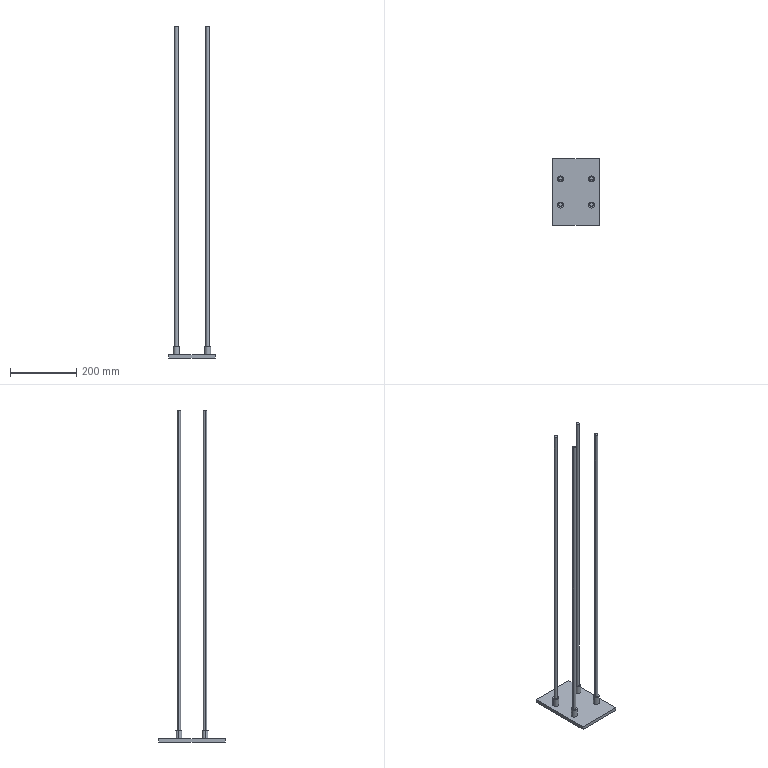Part | SolidWorks | features ICE 2, Extrusion 1 | 1 solid | 30 faces | box 140 x 200 x 1000 mm | volume 608611 mm3 | cylinder 16 | plane 14 | commonest cylinder face diameters 10 x8 18 x8
STEP:
#1=CARTESIAN_POINT('',(42.,-39.5,1000.));
#2=VERTEX_POINT('',#1);
#3=CARTESIAN_POINT('',(52.,-39.5,1000.));
#4=VERTEX_POINT('',#3);
#5=CARTESIAN_POINT('',(47.,-39.5,1000.));
#6=DIRECTION('',(0.,0.,-1.));
#7=DIRECTION('',(-1.,0.,0.));
#8=AXIS2_PLACEMENT_3D('',#5,#6,#7);
#9=CIRCLE('',#8,5.);
#10=EDGE_CURVE('',#2,#4,#9,.T.);
#11=ORIENTED_EDGE('',*,*,#10,.T.);
#12=CARTESIAN_POINT('',(52.,-39.5,35.));
#13=VERTEX_POINT('',#12);
#14=CARTESIAN_POINT('',(52.,-39.5,1000.));
#15=DIRECTION('',(0.,0.,-1.));
#16=VECTOR('',#15,1000.);
#17=LINE('',#14,#16);
#18=EDGE_CURVE('',#4,#13,#17,.T.);
#19=ORIENTED_EDGE('',*,*,#18,.T.);
#20=CARTESIAN_POINT('',(42.,-39.5,35.));
#21=VERTEX_POINT('',#20);
#22=CARTESIAN_POINT('',(47.,-39.5,35.));
#23=DIRECTION('',(0.,0.,1.));
#24=DIRECTION('',(1.,0.,0.));
#25=AXIS2_PLACEMENT_3D('',#22,#23,#24);
#26=CIRCLE('',#25,5.);
#27=EDGE_CURVE('',#13,#21,#26,.T.);
#28=ORIENTED_EDGE('',*,*,#27,.T.);
#29=CARTESIAN_POINT('',(42.,-39.5,1000.));
#30=DIRECTION('',(0.,0.,-1.));
#31=VECTOR('',#30,1000.);
#32=LINE('',#29,#31);
#33=EDGE_CURVE('',#2,#21,#32,.T.);
#34=ORIENTED_EDGE('',*,*,#33,.F.);
#35=EDGE_LOOP('',(#11,#19,#28,#34));
#36=FACE_OUTER_BOUND('',#35,.T.);
#37=CARTESIAN_POINT('',(47.,-39.5,1000.));
#38=DIRECTION('',(0.,0.,-1.));
#39=DIRECTION('',(-1.,0.,0.));
#40=AXIS2_PLACEMENT_3D('',#37,#38,#39);
#41=CYLINDRICAL_SURFACE('',#40,5.);
#42=ADVANCED_FACE('',(#36),#41,.T.);
#43=CARTESIAN_POINT('',(42.,39.5,1000.));
#44=VERTEX_POINT('',#43);
#45=CARTESIAN_POINT('',(52.,39.5,1000.));
#46=VERTEX_POINT('',#45);
#47=CARTESIAN_POINT('',(47.,39.5,1000.));
#48=DIRECTION('',(0.,0.,-1.));
#49=DIRECTION('',(-1.,0.,0.));
#50=AXIS2_PLACEMENT_3D('',#47,#48,#49);
#51=CIRCLE('',#50,5.);
#52=EDGE_CURVE('',#44,#46,#51,.T.);
#53=ORIENTED_EDGE('',*,*,#52,.T.);
#54=CARTESIAN_POINT('',(52.,39.5,35.));
#55=VERTEX_POINT('',#54);
#56=CARTESIAN_POINT('',(52.,39.5,1000.));
#57=DIRECTION('',(0.,0.,-1.));
#58=VECTOR('',#57,1000.);
#59=LINE('',#56,#58);
#60=EDGE_CURVE('',#46,#55,#59,.T.);
#61=ORIENTED_EDGE('',*,*,#60,.T.);
#62=CARTESIAN_POINT('',(42.,39.5,35.));
#63=VERTEX_POINT('',#62);
#64=CARTESIAN_POINT('',(47.,39.5,35.));
#65=DIRECTION('',(0.,0.,1.));
#66=DIRECTION('',(1.,0.,0.));
#67=AXIS2_PLACEMENT_3D('',#64,#65,#66);
#68=CIRCLE('',#67,5.);
#69=EDGE_CURVE('',#55,#63,#68,.T.);
#70=ORIENTED_EDGE('',*,*,#69,.T.);
#71=CARTESIAN_POINT('',(42.,39.5,1000.));
#72=DIRECTION('',(0.,0.,-1.));
#73=VECTOR('',#72,1000.);
#74=LINE('',#71,#73);
#75=EDGE_CURVE('',#44,#63,#74,.T.);
#76=ORIENTED_EDGE('',*,*,#75,.F.);
#77=EDGE_LOOP('',(#53,#61,#70,#76));
#78=FACE_OUTER_BOUND('',#77,.T.);
#79=CARTESIAN_POINT('',(47.,39.5,1000.));
#80=DIRECTION('',(0.,0.,-1.));
#81=DIRECTION('',(-1.,0.,0.));
#82=AXIS2_PLACEMENT_3D('',#79,#80,#81);
#83=CYLINDRICAL_SURFACE('',#82,5.);
#84=ADVANCED_FACE('',(#78),#83,.T.);
#85=CARTESIAN_POINT('',(-52.,-39.5,1000.));
#86=VERTEX_POINT('',#85);
#87=CARTESIAN_POINT('',(-42.,-39.5,1000.));
#88=VERTEX_POINT('',#87);
#89=CARTESIAN_POINT('',(-47.,-39.5,1000.));
#90=DIRECTION('',(0.,0.,-1.));
#91=DIRECTION('',(-1.,0.,0.));
#92=AXIS2_PLACEMENT_3D('',#89,#90,#91);
#93=CIRCLE('',#92,5.);
#94=EDGE_CURVE('',#86,#88,#93,.T.);
#95=ORIENTED_EDGE('',*,*,#94,.T.);
#96=CARTESIAN_POINT('',(-42.,-39.5,35.));
#97=VERTEX_POINT('',#96);
#98=CARTESIAN_POINT('',(-42.,-39.5,1000.));
#99=DIRECTION('',(0.,0.,-1.));
#100=VECTOR('',#99,1000.);
#101=LINE('',#98,#100);
#102=EDGE_CURVE('',#88,#97,#101,.T.);
#103=ORIENTED_EDGE('',*,*,#102,.T.);
#104=CARTESIAN_POINT('',(-52.,-39.5,35.));
#105=VERTEX_POINT('',#104);
#106=CARTESIAN_POINT('',(-47.,-39.5,35.));
#107=DIRECTION('',(0.,0.,1.));
#108=DIRECTION('',(1.,0.,0.));
#109=AXIS2_PLACEMENT_3D('',#106,#107,#108);
#110=CIRCLE('',#109,5.);
#111=EDGE_CURVE('',#97,#105,#110,.T.);
#112=ORIENTED_EDGE('',*,*,#111,.T.);
#113=CARTESIAN_POINT('',(-52.,-39.5,1000.));
#114=DIRECTION('',(0.,0.,-1.));
#115=VECTOR('',#114,1000.);
#116=LINE('',#113,#115);
#117=EDGE_CURVE('',#86,#105,#116,.T.);
#118=ORIENTED_EDGE('',*,*,#117,.F.);
#119=EDGE_LOOP('',(#95,#103,#112,#118));
#120=FACE_OUTER_BOUND('',#119,.T.);
#121=CARTESIAN_POINT('',(-47.,-39.5,1000.));
#122=DIRECTION('',(0.,0.,-1.));
#123=DIRECTION('',(-1.,0.,0.));
#124=AXIS2_PLACEMENT_3D('',#121,#122,#123);
#125=CYLINDRICAL_SURFACE('',#124,5.);
#126=ADVANCED_FACE('',(#120),#125,.T.);
#127=CARTESIAN_POINT('',(-52.,39.5,1000.));
#128=VERTEX_POINT('',#127);
#129=CARTESIAN_POINT('',(-42.,39.5,1000.));
#130=VERTEX_POINT('',#129);
#131=CARTESIAN_POINT('',(-47.,39.5,1000.));
#132=DIRECTION('',(0.,0.,-1.));
#133=DIRECTION('',(-1.,0.,0.));
#134=AXIS2_PLACEMENT_3D('',#131,#132,#133);
#135=CIRCLE('',#134,5.);
#136=EDGE_CURVE('',#128,#130,#135,.T.);
#137=ORIENTED_EDGE('',*,*,#136,.T.);
#138=CARTESIAN_POINT('',(-42.,39.5,35.));
#139=VERTEX_POINT('',#138);
#140=CARTESIAN_POINT('',(-42.,39.5,1000.));
#141=DIRECTION('',(0.,0.,-1.));
#142=VECTOR('',#141,1000.);
#143=LINE('',#140,#142);
#144=EDGE_CURVE('',#130,#139,#143,.T.);
#145=ORIENTED_EDGE('',*,*,#144,.T.);
#146=CARTESIAN_POINT('',(-52.,39.5,35.));
#147=VERTEX_POINT('',#146);
#148=CARTESIAN_POINT('',(-47.,39.5,35.));
#149=DIRECTION('',(0.,0.,1.));
#150=DIRECTION('',(1.,0.,0.));
#151=AXIS2_PLACEMENT_3D('',#148,#149,#150);
#152=CIRCLE('',#151,5.);
#153=EDGE_CURVE('',#139,#147,#152,.T.);
#154=ORIENTED_EDGE('',*,*,#153,.T.);
#155=CARTESIAN_POINT('',(-52.,39.5,1000.));
#156=DIRECTION('',(0.,0.,-1.));
#157=VECTOR('',#156,1000.);
#158=LINE('',#155,#157);
#159=EDGE_CURVE('',#128,#147,#158,.T.);
#160=ORIENTED_EDGE('',*,*,#159,.F.);
#161=EDGE_LOOP('',(#137,#145,#154,#160));
#162=FACE_OUTER_BOUND('',#161,.T.);
#163=CARTESIAN_POINT('',(-47.,39.5,1000.));
#164=DIRECTION('',(0.,0.,-1.));
#165=DIRECTION('',(-1.,0.,0.));
#166=AXIS2_PLACEMENT_3D('',#163,#164,#165);
#167=CYLINDRICAL_SURFACE('',#166,5.);
#168=ADVANCED_FACE('',(#162),#167,.T.);
#169=CARTESIAN_POINT('',(-38.,39.5,35.));
#170=VERTEX_POINT('',#169);
#171=CARTESIAN_POINT('',(-56.,39.5,35.));
#172=VERTEX_POINT('',#171);
#173=CARTESIAN_POINT('',(-47.,39.5,35.));
#174=DIRECTION('',(0.,0.,1.));
#175=DIRECTION('',(1.,0.,0.));
#176=AXIS2_PLACEMENT_3D('',#173,#174,#175);
#177=CIRCLE('',#176,9.);
#178=EDGE_CURVE('',#170,#172,#177,.T.);
#179=ORIENTED_EDGE('',*,*,#178,.F.);
#180=CARTESIAN_POINT('',(-38.,39.5,10.));
#181=VERTEX_POINT('',#180);
#182=CARTESIAN_POINT('',(-38.,39.5,35.));
#183=DIRECTION('',(0.,0.,-1.));
#184=VECTOR('',#183,1000.);
#185=LINE('',#182,#184);
#186=EDGE_CURVE('',#170,#181,#185,.T.);
#187=ORIENTED_EDGE('',*,*,#186,.T.);
#188=CARTESIAN_POINT('',(-56.,39.5,10.));
#189=VERTEX_POINT('',#188);
#190=CARTESIAN_POINT('',(-47.,39.5,10.));
#191=DIRECTION('',(0.,0.,1.));
#192=DIRECTION('',(1.,0.,0.));
#193=AXIS2_PLACEMENT_3D('',#190,#191,#192);
#194=CIRCLE('',#193,9.);
#195=EDGE_CURVE('',#181,#189,#194,.T.);
#196=ORIENTED_EDGE('',*,*,#195,.T.);
#197=CARTESIAN_POINT('',(-56.,39.5,35.));
#198=DIRECTION('',(0.,0.,-1.));
#199=VECTOR('',#198,1000.);
#200=LINE('',#197,#199);
#201=EDGE_CURVE('',#172,#189,#200,.T.);
#202=ORIENTED_EDGE('',*,*,#201,.F.);
#203=EDGE_LOOP('',(#179,#187,#196,#202));
#204=FACE_OUTER_BOUND('',#203,.T.);
#205=CARTESIAN_POINT('',(-47.,39.5,35.));
#206=DIRECTION('',(0.,0.,-1.));
#207=DIRECTION('',(-1.,0.,0.));
#208=AXIS2_PLACEMENT_3D('',#205,#206,#207);
#209=CYLINDRICAL_SURFACE('',#208,9.);
#210=ADVANCED_FACE('',(#204),#209,.T.);
#211=CARTESIAN_POINT('',(-38.,-39.5,35.));
#212=VERTEX_POINT('',#211);
#213=CARTESIAN_POINT('',(-56.,-39.5,35.));
#214=VERTEX_POINT('',#213);
#215=CARTESIAN_POINT('',(-47.,-39.5,35.));
#216=DIRECTION('',(0.,0.,1.));
#217=DIRECTION('',(1.,0.,0.));
#218=AXIS2_PLACEMENT_3D('',#215,#216,#217);
#219=CIRCLE('',#218,9.);
#220=EDGE_CURVE('',#212,#214,#219,.T.);
#221=ORIENTED_EDGE('',*,*,#220,.F.);
#222=CARTESIAN_POINT('',(-38.,-39.5,10.));
#223=VERTEX_POINT('',#222);
#224=CARTESIAN_POINT('',(-38.,-39.5,35.));
#225=DIRECTION('',(0.,0.,-1.));
#226=VECTOR('',#225,1000.);
#227=LINE('',#224,#226);
#228=EDGE_CURVE('',#212,#223,#227,.T.);
#229=ORIENTED_EDGE('',*,*,#228,.T.);
#230=CARTESIAN_POINT('',(-56.,-39.5,10.));
#231=VERTEX_POINT('',#230);
#232=CARTESIAN_POINT('',(-47.,-39.5,10.));
#233=DIRECTION('',(0.,0.,1.));
#234=DIRECTION('',(1.,0.,0.));
#235=AXIS2_PLACEMENT_3D('',#232,#233,#234);
#236=CIRCLE('',#235,9.);
#237=EDGE_CURVE('',#223,#231,#236,.T.);
#238=ORIENTED_EDGE('',*,*,#237,.T.);
#239=CARTESIAN_POINT('',(-56.,-39.5,35.));
#240=DIRECTION('',(0.,0.,-1.));
#241=VECTOR('',#240,1000.);
#242=LINE('',#239,#241);
#243=EDGE_CURVE('',#214,#231,#242,.T.);
#244=ORIENTED_EDGE('',*,*,#243,.F.);
#245=EDGE_LOOP('',(#221,#229,#238,#244));
#246=FACE_OUTER_BOUND('',#245,.T.);
#247=CARTESIAN_POINT('',(-47.,-39.5,35.));
#248=DIRECTION('',(0.,0.,-1.));
#249=DIRECTION('',(-1.,0.,0.));
#250=AXIS2_PLACEMENT_3D('',#247,#248,#249);
#251=CYLINDRICAL_SURFACE('',#250,9.);
#252=ADVANCED_FACE('',(#246),#251,.T.);
#253=CARTESIAN_POINT('',(56.,39.5,35.));
#254=VERTEX_POINT('',#253);
#255=CARTESIAN_POINT('',(38.,39.5,35.));
#256=VERTEX_POINT('',#255);
#257=CARTESIAN_POINT('',(47.,39.5,35.));
#258=DIRECTION('',(0.,0.,1.));
#259=DIRECTION('',(1.,0.,0.));
#260=AXIS2_PLACEMENT_3D('',#257,#258,#259);
#261=CIRCLE('',#260,9.);
#262=EDGE_CURVE('',#254,#256,#261,.T.);
#263=ORIENTED_EDGE('',*,*,#262,.F.);
#264=CARTESIAN_POINT('',(56.,39.5,10.));
#265=VERTEX_POINT('',#264);
#266=CARTESIAN_POINT('',(56.,39.5,35.));
#267=DIRECTION('',(0.,0.,-1.));
#268=VECTOR('',#267,1000.);
#269=LINE('',#266,#268);
#270=EDGE_CURVE('',#254,#265,#269,.T.);
#271=ORIENTED_EDGE('',*,*,#270,.T.);
#272=CARTESIAN_POINT('',(38.,39.5,10.));
#273=VERTEX_POINT('',#272);
#274=CARTESIAN_POINT('',(47.,39.5,10.));
#275=DIRECTION('',(0.,0.,1.));
#276=DIRECTION('',(1.,0.,0.));
#277=AXIS2_PLACEMENT_3D('',#274,#275,#276);
#278=CIRCLE('',#277,9.);
#279=EDGE_CURVE('',#265,#273,#278,.T.);
#280=ORIENTED_EDGE('',*,*,#279,.T.);
#281=CARTESIAN_POINT('',(38.,39.5,35.));
#282=DIRECTION('',(0.,0.,-1.));
#283=VECTOR('',#282,1000.);
#284=LINE('',#281,#283);
#285=EDGE_CURVE('',#256,#273,#284,.T.);
#286=ORIENTED_EDGE('',*,*,#285,.F.);
#287=EDGE_LOOP('',(#263,#271,#280,#286));
#288=FACE_OUTER_BOUND('',#287,.T.);
#289=CARTESIAN_POINT('',(47.,39.5,35.));
#290=DIRECTION('',(0.,0.,-1.));
#291=DIRECTION('',(-1.,0.,0.));
#292=AXIS2_PLACEMENT_3D('',#289,#290,#291);
#293=CYLINDRICAL_SURFACE('',#292,9.);
#294=ADVANCED_FACE('',(#288),#293,.T.);
#295=CARTESIAN_POINT('',(56.,-39.5,35.));
#296=VERTEX_POINT('',#295);
#297=CARTESIAN_POINT('',(38.,-39.5,35.));
#298=VERTEX_POINT('',#297);
#299=CARTESIAN_POINT('',(47.,-39.5,35.));
#300=DIRECTION('',(0.,0.,1.));
#301=DIRECTION('',(1.,0.,0.));
#302=AXIS2_PLACEMENT_3D('',#299,#300,#301);
#303=CIRCLE('',#302,9.);
#304=EDGE_CURVE('',#296,#298,#303,.T.);
#305=ORIENTED_EDGE('',*,*,#304,.F.);
#306=CARTESIAN_POINT('',(56.,-39.5,10.));
#307=VERTEX_POINT('',#306);
#308=CARTESIAN_POINT('',(56.,-39.5,35.));
#309=DIRECTION('',(0.,0.,-1.));
#310=VECTOR('',#309,1000.);
#311=LINE('',#308,#310);
#312=EDGE_CURVE('',#296,#307,#311,.T.);
#313=ORIENTED_EDGE('',*,*,#312,.T.);
#314=CARTESIAN_POINT('',(38.,-39.5,10.));
#315=VERTEX_POINT('',#314);
#316=CARTESIAN_POINT('',(47.,-39.5,10.));
#317=DIRECTION('',(0.,0.,1.));
#318=DIRECTION('',(1.,0.,0.));
#319=AXIS2_PLACEMENT_3D('',#316,#317,#318);
#320=CIRCLE('',#319,9.);
#321=EDGE_CURVE('',#307,#315,#320,.T.);
#322=ORIENTED_EDGE('',*,*,#321,.T.);
#323=CARTESIAN_POINT('',(38.,-39.5,35.));
#324=DIRECTION('',(0.,0.,-1.));
#325=VECTOR('',#324,1000.);
#326=LINE('',#323,#325);
#327=EDGE_CURVE('',#298,#315,#326,.T.);
#328=ORIENTED_EDGE('',*,*,#327,.F.);
#329=EDGE_LOOP('',(#305,#313,#322,#328));
#330=FACE_OUTER_BOUND('',#329,.T.);
#331=CARTESIAN_POINT('',(47.,-39.5,35.));
#332=DIRECTION('',(0.,0.,-1.));
#333=DIRECTION('',(-1.,0.,0.));
#334=AXIS2_PLACEMENT_3D('',#331,#332,#333);
#335=CYLINDRICAL_SURFACE('',#334,9.);
#336=ADVANCED_FACE('',(#330),#335,.T.);
#337=CARTESIAN_POINT('',(47.,-39.5,10.));
#338=DIRECTION('',(0.,0.,1.));
#339=DIRECTION('',(1.,0.,0.));
#340=AXIS2_PLACEMENT_3D('',#337,#338,#339);
#341=CIRCLE('',#340,9.);
#342=EDGE_CURVE('',#315,#307,#341,.T.);
#343=ORIENTED_EDGE('',*,*,#342,.F.);
#344=ORIENTED_EDGE('',*,*,#321,.F.);
#345=EDGE_LOOP('',(#343,#344));
#346=FACE_BOUND('',#345,.T.);
#347=CARTESIAN_POINT('',(-47.,39.5,10.));
#348=DIRECTION('',(0.,0.,1.));
#349=DIRECTION('',(1.,0.,0.));
#350=AXIS2_PLACEMENT_3D('',#347,#348,#349);
#351=CIRCLE('',#350,9.);
#352=EDGE_CURVE('',#189,#181,#351,.T.);
#353=ORIENTED_EDGE('',*,*,#352,.F.);
#354=ORIENTED_EDGE('',*,*,#195,.F.);
#355=EDGE_LOOP('',(#353,#354));
#356=FACE_BOUND('',#355,.T.);
#357=CARTESIAN_POINT('',(70.,-100.,10.));
#358=VERTEX_POINT('',#357);
#359=CARTESIAN_POINT('',(70.,100.,10.));
#360=VERTEX_POINT('',#359);
#361=CARTESIAN_POINT('',(70.,100.,10.));
#362=DIRECTION('',(0.,1.,0.));
#363=VECTOR('',#362,1000.);
#364=LINE('',#361,#363);
#365=EDGE_CURVE('',#358,#360,#364,.T.);
#366=ORIENTED_EDGE('',*,*,#365,.T.);
#367=CARTESIAN_POINT('',(-70.,100.,10.));
#368=VERTEX_POINT('',#367);
#369=CARTESIAN_POINT('',(-70.,100.,10.));
#370=DIRECTION('',(-1.,0.,0.));
#371=VECTOR('',#370,1000.);
#372=LINE('',#369,#371);
#373=EDGE_CURVE('',#360,#368,#372,.T.);
#374=ORIENTED_EDGE('',*,*,#373,.T.);
#375=CARTESIAN_POINT('',(-70.,-100.,10.));
#376=VERTEX_POINT('',#375);
#377=CARTESIAN_POINT('',(-70.,100.,10.));
#378=DIRECTION('',(0.,-1.,0.));
#379=VECTOR('',#378,1000.);
#380=LINE('',#377,#379);
#381=EDGE_CURVE('',#368,#376,#380,.T.);
#382=ORIENTED_EDGE('',*,*,#381,.T.);
#383=CARTESIAN_POINT('',(-70.,-100.,10.));
#384=DIRECTION('',(1.,0.,0.));
#385=VECTOR('',#384,1000.);
#386=LINE('',#383,#385);
#387=EDGE_CURVE('',#376,#358,#386,.T.);
#388=ORIENTED_EDGE('',*,*,#387,.T.);
#389=EDGE_LOOP('',(#366,#374,#382,#388));
#390=FACE_OUTER_BOUND('',#389,.T.);
#391=CARTESIAN_POINT('',(47.,39.5,10.));
#392=DIRECTION('',(0.,0.,1.));
#393=DIRECTION('',(1.,0.,0.));
#394=AXIS2_PLACEMENT_3D('',#391,#392,#393);
#395=CIRCLE('',#394,9.);
#396=EDGE_CURVE('',#273,#265,#395,.T.);
#397=ORIENTED_EDGE('',*,*,#396,.F.);
#398=ORIENTED_EDGE('',*,*,#279,.F.);
#399=EDGE_LOOP('',(#397,#398));
#400=FACE_BOUND('',#399,.T.);
#401=CARTESIAN_POINT('',(-47.,-39.5,10.));
#402=DIRECTION('',(0.,0.,1.));
#403=DIRECTION('',(1.,0.,0.));
#404=AXIS2_PLACEMENT_3D('',#401,#402,#403);
#405=CIRCLE('',#404,9.);
#406=EDGE_CURVE('',#231,#223,#405,.T.);
#407=ORIENTED_EDGE('',*,*,#406,.F.);
#408=ORIENTED_EDGE('',*,*,#237,.F.);
#409=EDGE_LOOP('',(#407,#408));
#410=FACE_BOUND('',#409,.T.);
#411=CARTESIAN_POINT('',(0.,0.,10.));
#412=DIRECTION('',(0.,0.,1.));
#413=DIRECTION('',(1.,0.,0.));
#414=AXIS2_PLACEMENT_3D('',#411,#412,#413);
#415=PLANE('',#414);
#416=ADVANCED_FACE('',(#346,#356,#390,#400,#410),#415,.T.);
#417=CARTESIAN_POINT('',(70.,-100.,0.));
#418=VERTEX_POINT('',#417);
#419=CARTESIAN_POINT('',(70.,100.,0.));
#420=VERTEX_POINT('',#419);
#421=CARTESIAN_POINT('',(70.,100.,0.));
#422=DIRECTION('',(0.,1.,0.));
#423=VECTOR('',#422,1000.);
#424=LINE('',#421,#423);
#425=EDGE_CURVE('',#418,#420,#424,.T.);
#426=ORIENTED_EDGE('',*,*,#425,.F.);
#427=CARTESIAN_POINT('',(-70.,-100.,0.));
#428=VERTEX_POINT('',#427);
#429=CARTESIAN_POINT('',(-70.,-100.,0.));
#430=DIRECTION('',(1.,0.,0.));
#431=VECTOR('',#430,1000.);
#432=LINE('',#429,#431);
#433=EDGE_CURVE('',#428,#418,#432,.T.);
#434=ORIENTED_EDGE('',*,*,#433,.F.);
#435=CARTESIAN_POINT('',(-70.,100.,0.));
#436=VERTEX_POINT('',#435);
#437=CARTESIAN_POINT('',(-70.,100.,0.));
#438=DIRECTION('',(0.,-1.,0.));
#439=VECTOR('',#438,1000.);
#440=LINE('',#437,#439);
#441=EDGE_CURVE('',#436,#428,#440,.T.);
#442=ORIENTED_EDGE('',*,*,#441,.F.);
#443=CARTESIAN_POINT('',(-70.,100.,0.));
#444=DIRECTION('',(-1.,0.,0.));
#445=VECTOR('',#444,1000.);
#446=LINE('',#443,#445);
#447=EDGE_CURVE('',#420,#436,#446,.T.);
#448=ORIENTED_EDGE('',*,*,#447,.F.);
#449=EDGE_LOOP('',(#426,#434,#442,#448));
#450=FACE_OUTER_BOUND('',#449,.T.);
#451=CARTESIAN_POINT('',(0.,0.,0.));
#452=DIRECTION('',(0.,0.,1.));
#453=DIRECTION('',(1.,0.,0.));
#454=AXIS2_PLACEMENT_3D('',#451,#452,#453);
#455=PLANE('',#454);
#456=ADVANCED_FACE('',(#450),#455,.F.);
#457=ORIENTED_EDGE('',*,*,#425,.T.);
#458=CARTESIAN_POINT('',(70.,100.,10.));
#459=DIRECTION('',(0.,0.,-1.));
#460=VECTOR('',#459,1000.);
#461=LINE('',#458,#460);
#462=EDGE_CURVE('',#360,#420,#461,.T.);
#463=ORIENTED_EDGE('',*,*,#462,.F.);
#464=ORIENTED_EDGE('',*,*,#365,.F.);
#465=CARTESIAN_POINT('',(70.,-100.,10.));
#466=DIRECTION('',(0.,0.,-1.));
#467=VECTOR('',#466,1000.);
#468=LINE('',#465,#467);
#469=EDGE_CURVE('',#358,#418,#468,.T.);
#470=ORIENTED_EDGE('',*,*,#469,.T.);
#471=EDGE_LOOP('',(#457,#463,#464,#470));
#472=FACE_OUTER_BOUND('',#471,.T.);
#473=CARTESIAN_POINT('',(70.,100.,10.));
#474=DIRECTION('',(-1.,0.,0.));
#475=DIRECTION('',(0.,-1.,0.));
#476=AXIS2_PLACEMENT_3D('',#473,#474,#475);
#477=PLANE('',#476);
#478=ADVANCED_FACE('',(#472),#477,.F.);
#479=ORIENTED_EDGE('',*,*,#447,.T.);
#480=CARTESIAN_POINT('',(-70.,100.,10.));
#481=DIRECTION('',(0.,0.,-1.));
#482=VECTOR('',#481,1000.);
#483=LINE('',#480,#482);
#484=EDGE_CURVE('',#368,#436,#483,.T.);
#485=ORIENTED_EDGE('',*,*,#484,.F.);
#486=ORIENTED_EDGE('',*,*,#373,.F.);
#487=ORIENTED_EDGE('',*,*,#462,.T.);
#488=EDGE_LOOP('',(#479,#485,#486,#487));
#489=FACE_OUTER_BOUND('',#488,.T.);
#490=CARTESIAN_POINT('',(-70.,100.,10.));
#491=DIRECTION('',(0.,-1.,0.));
#492=DIRECTION('',(1.,0.,0.));
#493=AXIS2_PLACEMENT_3D('',#490,#491,#492);
#494=PLANE('',#493);
#495=ADVANCED_FACE('',(#489),#494,.F.);
#496=ORIENTED_EDGE('',*,*,#441,.T.);
#497=CARTESIAN_POINT('',(-70.,-100.,10.));
#498=DIRECTION('',(0.,0.,-1.));
#499=VECTOR('',#498,1000.);
#500=LINE('',#497,#499);
#501=EDGE_CURVE('',#376,#428,#500,.T.);
#502=ORIENTED_EDGE('',*,*,#501,.F.);
#503=ORIENTED_EDGE('',*,*,#381,.F.);
#504=ORIENTED_EDGE('',*,*,#484,.T.);
#505=EDGE_LOOP('',(#496,#502,#503,#504));
#506=FACE_OUTER_BOUND('',#505,.T.);
#507=CARTESIAN_POINT('',(-70.,100.,10.));
#508=DIRECTION('',(1.,0.,0.));
#509=DIRECTION('',(0.,1.,0.));
#510=AXIS2_PLACEMENT_3D('',#507,#508,#509);
#511=PLANE('',#510);
#512=ADVANCED_FACE('',(#506),#511,.F.);
#513=ORIENTED_EDGE('',*,*,#433,.T.);
#514=ORIENTED_EDGE('',*,*,#469,.F.);
#515=ORIENTED_EDGE('',*,*,#387,.F.);
#516=ORIENTED_EDGE('',*,*,#501,.T.);
#517=EDGE_LOOP('',(#513,#514,#515,#516));
#518=FACE_OUTER_BOUND('',#517,.T.);
#519=CARTESIAN_POINT('',(-70.,-100.,10.));
#520=DIRECTION('',(0.,1.,0.));
#521=DIRECTION('',(0.,0.,1.));
#522=AXIS2_PLACEMENT_3D('',#519,#520,#521);
#523=PLANE('',#522);
#524=ADVANCED_FACE('',(#518),#523,.F.);
#525=CARTESIAN_POINT('',(47.,-39.5,35.));
#526=DIRECTION('',(0.,0.,1.));
#527=DIRECTION('',(1.,0.,0.));
#528=AXIS2_PLACEMENT_3D('',#525,#526,#527);
#529=CIRCLE('',#528,9.);
#530=EDGE_CURVE('',#298,#296,#529,.T.);
#531=ORIENTED_EDGE('',*,*,#530,.T.);
#532=ORIENTED_EDGE('',*,*,#304,.T.);
#533=EDGE_LOOP('',(#531,#532));
#534=FACE_OUTER_BOUND('',#533,.T.);
#535=CARTESIAN_POINT('',(47.,-39.5,35.));
#536=DIRECTION('',(0.,0.,1.));
#537=DIRECTION('',(1.,0.,0.));
#538=AXIS2_PLACEMENT_3D('',#535,#536,#537);
#539=CIRCLE('',#538,5.);
#540=EDGE_CURVE('',#21,#13,#539,.T.);
#541=ORIENTED_EDGE('',*,*,#540,.F.);
#542=ORIENTED_EDGE('',*,*,#27,.F.);
#543=EDGE_LOOP('',(#541,#542));
#544=FACE_BOUND('',#543,.T.);
#545=CARTESIAN_POINT('',(47.,-39.5,35.));
#546=DIRECTION('',(0.,0.,1.));
#547=DIRECTION('',(1.,0.,0.));
#548=AXIS2_PLACEMENT_3D('',#545,#546,#547);
#549=PLANE('',#548);
#550=ADVANCED_FACE('',(#534,#544),#549,.T.);
#551=ORIENTED_EDGE('',*,*,#312,.F.);
#552=ORIENTED_EDGE('',*,*,#530,.F.);
#553=ORIENTED_EDGE('',*,*,#327,.T.);
#554=ORIENTED_EDGE('',*,*,#342,.T.);
#555=EDGE_LOOP('',(#551,#552,#553,#554));
#556=FACE_OUTER_BOUND('',#555,.T.);
#557=CARTESIAN_POINT('',(47.,-39.5,35.));
#558=DIRECTION('',(0.,0.,-1.));
#559=DIRECTION('',(-1.,0.,0.));
#560=AXIS2_PLACEMENT_3D('',#557,#558,#559);
#561=CYLINDRICAL_SURFACE('',#560,9.);
#562=ADVANCED_FACE('',(#556),#561,.T.);
#563=CARTESIAN_POINT('',(47.,39.5,35.));
#564=DIRECTION('',(0.,0.,1.));
#565=DIRECTION('',(1.,0.,0.));
#566=AXIS2_PLACEMENT_3D('',#563,#564,#565);
#567=CIRCLE('',#566,9.);
#568=EDGE_CURVE('',#256,#254,#567,.T.);
#569=ORIENTED_EDGE('',*,*,#568,.T.);
#570=ORIENTED_EDGE('',*,*,#262,.T.);
#571=EDGE_LOOP('',(#569,#570));
#572=FACE_OUTER_BOUND('',#571,.T.);
#573=CARTESIAN_POINT('',(47.,39.5,35.));
#574=DIRECTION('',(0.,0.,1.));
#575=DIRECTION('',(1.,0.,0.));
#576=AXIS2_PLACEMENT_3D('',#573,#574,#575);
#577=CIRCLE('',#576,5.);
#578=EDGE_CURVE('',#63,#55,#577,.T.);
#579=ORIENTED_EDGE('',*,*,#578,.F.);
#580=ORIENTED_EDGE('',*,*,#69,.F.);
#581=EDGE_LOOP('',(#579,#580));
#582=FACE_BOUND('',#581,.T.);
#583=CARTESIAN_POINT('',(47.,39.5,35.));
#584=DIRECTION('',(0.,0.,1.));
#585=DIRECTION('',(1.,0.,0.));
#586=AXIS2_PLACEMENT_3D('',#583,#584,#585);
#587=PLANE('',#586);
#588=ADVANCED_FACE('',(#572,#582),#587,.T.);
#589=ORIENTED_EDGE('',*,*,#270,.F.);
#590=ORIENTED_EDGE('',*,*,#568,.F.);
#591=ORIENTED_EDGE('',*,*,#285,.T.);
#592=ORIENTED_EDGE('',*,*,#396,.T.);
#593=EDGE_LOOP('',(#589,#590,#591,#592));
#594=FACE_OUTER_BOUND('',#593,.T.);
#595=CARTESIAN_POINT('',(47.,39.5,35.));
#596=DIRECTION('',(0.,0.,-1.));
#597=DIRECTION('',(-1.,0.,0.));
#598=AXIS2_PLACEMENT_3D('',#595,#596,#597);
#599=CYLINDRICAL_SURFACE('',#598,9.);
#600=ADVANCED_FACE('',(#594),#599,.T.);
#601=CARTESIAN_POINT('',(-47.,-39.5,35.));
#602=DIRECTION('',(0.,0.,1.));
#603=DIRECTION('',(1.,0.,0.));
#604=AXIS2_PLACEMENT_3D('',#601,#602,#603);
#605=CIRCLE('',#604,9.);
#606=EDGE_CURVE('',#214,#212,#605,.T.);
#607=ORIENTED_EDGE('',*,*,#606,.T.);
#608=ORIENTED_EDGE('',*,*,#220,.T.);
#609=EDGE_LOOP('',(#607,#608));
#610=FACE_OUTER_BOUND('',#609,.T.);
#611=CARTESIAN_POINT('',(-47.,-39.5,35.));
#612=DIRECTION('',(0.,0.,1.));
#613=DIRECTION('',(1.,0.,0.));
#614=AXIS2_PLACEMENT_3D('',#611,#612,#613);
#615=CIRCLE('',#614,5.);
#616=EDGE_CURVE('',#105,#97,#615,.T.);
#617=ORIENTED_EDGE('',*,*,#616,.F.);
#618=ORIENTED_EDGE('',*,*,#111,.F.);
#619=EDGE_LOOP('',(#617,#618));
#620=FACE_BOUND('',#619,.T.);
#621=CARTESIAN_POINT('',(-47.,-39.5,35.));
#622=DIRECTION('',(0.,0.,1.));
#623=DIRECTION('',(1.,0.,0.));
#624=AXIS2_PLACEMENT_3D('',#621,#622,#623);
#625=PLANE('',#624);
#626=ADVANCED_FACE('',(#610,#620),#625,.T.);
#627=ORIENTED_EDGE('',*,*,#228,.F.);
#628=ORIENTED_EDGE('',*,*,#606,.F.);
#629=ORIENTED_EDGE('',*,*,#243,.T.);
#630=ORIENTED_EDGE('',*,*,#406,.T.);
#631=EDGE_LOOP('',(#627,#628,#629,#630));
#632=FACE_OUTER_BOUND('',#631,.T.);
#633=CARTESIAN_POINT('',(-47.,-39.5,35.));
#634=DIRECTION('',(0.,0.,-1.));
#635=DIRECTION('',(-1.,0.,0.));
#636=AXIS2_PLACEMENT_3D('',#633,#634,#635);
#637=CYLINDRICAL_SURFACE('',#636,9.);
#638=ADVANCED_FACE('',(#632),#637,.T.);
#639=CARTESIAN_POINT('',(-47.,39.5,35.));
#640=DIRECTION('',(0.,0.,1.));
#641=DIRECTION('',(1.,0.,0.));
#642=AXIS2_PLACEMENT_3D('',#639,#640,#641);
#643=CIRCLE('',#642,9.);
#644=EDGE_CURVE('',#172,#170,#643,.T.);
#645=ORIENTED_EDGE('',*,*,#644,.T.);
#646=ORIENTED_EDGE('',*,*,#178,.T.);
#647=EDGE_LOOP('',(#645,#646));
#648=FACE_OUTER_BOUND('',#647,.T.);
#649=CARTESIAN_POINT('',(-47.,39.5,35.));
#650=DIRECTION('',(0.,0.,1.));
#651=DIRECTION('',(1.,0.,0.));
#652=AXIS2_PLACEMENT_3D('',#649,#650,#651);
#653=CIRCLE('',#652,5.);
#654=EDGE_CURVE('',#147,#139,#653,.T.);
#655=ORIENTED_EDGE('',*,*,#654,.F.);
#656=ORIENTED_EDGE('',*,*,#153,.F.);
#657=EDGE_LOOP('',(#655,#656));
#658=FACE_BOUND('',#657,.T.);
#659=CARTESIAN_POINT('',(-47.,39.5,35.));
#660=DIRECTION('',(0.,0.,1.));
#661=DIRECTION('',(1.,0.,0.));
#662=AXIS2_PLACEMENT_3D('',#659,#660,#661);
#663=PLANE('',#662);
#664=ADVANCED_FACE('',(#648,#658),#663,.T.);
#665=ORIENTED_EDGE('',*,*,#186,.F.);
#666=ORIENTED_EDGE('',*,*,#644,.F.);
#667=ORIENTED_EDGE('',*,*,#201,.T.);
#668=ORIENTED_EDGE('',*,*,#352,.T.);
#669=EDGE_LOOP('',(#665,#666,#667,#668));
#670=FACE_OUTER_BOUND('',#669,.T.);
#671=CARTESIAN_POINT('',(-47.,39.5,35.));
#672=DIRECTION('',(0.,0.,-1.));
#673=DIRECTION('',(-1.,0.,0.));
#674=AXIS2_PLACEMENT_3D('',#671,#672,#673);
#675=CYLINDRICAL_SURFACE('',#674,9.);
#676=ADVANCED_FACE('',(#670),#675,.T.);
#677=ORIENTED_EDGE('',*,*,#136,.F.);
#678=CARTESIAN_POINT('',(-47.,39.5,1000.));
#679=DIRECTION('',(0.,0.,-1.));
#680=DIRECTION('',(-1.,0.,0.));
#681=AXIS2_PLACEMENT_3D('',#678,#679,#680);
#682=CIRCLE('',#681,5.);
#683=EDGE_CURVE('',#130,#128,#682,.T.);
#684=ORIENTED_EDGE('',*,*,#683,.F.);
#685=EDGE_LOOP('',(#677,#684));
#686=FACE_OUTER_BOUND('',#685,.T.);
#687=CARTESIAN_POINT('',(-47.,39.5,1000.));
#688=DIRECTION('',(0.,0.,-1.));
#689=DIRECTION('',(-1.,0.,0.));
#690=AXIS2_PLACEMENT_3D('',#687,#688,#689);
#691=PLANE('',#690);
#692=ADVANCED_FACE('',(#686),#691,.F.);
#693=ORIENTED_EDGE('',*,*,#144,.F.);
#694=ORIENTED_EDGE('',*,*,#683,.T.);
#695=ORIENTED_EDGE('',*,*,#159,.T.);
#696=ORIENTED_EDGE('',*,*,#654,.T.);
#697=EDGE_LOOP('',(#693,#694,#695,#696));
#698=FACE_OUTER_BOUND('',#697,.T.);
#699=CARTESIAN_POINT('',(-47.,39.5,1000.));
#700=DIRECTION('',(0.,0.,-1.));
#701=DIRECTION('',(-1.,0.,0.));
#702=AXIS2_PLACEMENT_3D('',#699,#700,#701);
#703=CYLINDRICAL_SURFACE('',#702,5.);
#704=ADVANCED_FACE('',(#698),#703,.T.);
#705=ORIENTED_EDGE('',*,*,#94,.F.);
#706=CARTESIAN_POINT('',(-47.,-39.5,1000.));
#707=DIRECTION('',(0.,0.,-1.));
#708=DIRECTION('',(-1.,0.,0.));
#709=AXIS2_PLACEMENT_3D('',#706,#707,#708);
#710=CIRCLE('',#709,5.);
#711=EDGE_CURVE('',#88,#86,#710,.T.);
#712=ORIENTED_EDGE('',*,*,#711,.F.);
#713=EDGE_LOOP('',(#705,#712));
#714=FACE_OUTER_BOUND('',#713,.T.);
#715=CARTESIAN_POINT('',(-47.,-39.5,1000.));
#716=DIRECTION('',(0.,0.,-1.));
#717=DIRECTION('',(-1.,0.,0.));
#718=AXIS2_PLACEMENT_3D('',#715,#716,#717);
#719=PLANE('',#718);
#720=ADVANCED_FACE('',(#714),#719,.F.);
#721=ORIENTED_EDGE('',*,*,#102,.F.);
#722=ORIENTED_EDGE('',*,*,#711,.T.);
#723=ORIENTED_EDGE('',*,*,#117,.T.);
#724=ORIENTED_EDGE('',*,*,#616,.T.);
#725=EDGE_LOOP('',(#721,#722,#723,#724));
#726=FACE_OUTER_BOUND('',#725,.T.);
#727=CARTESIAN_POINT('',(-47.,-39.5,1000.));
#728=DIRECTION('',(0.,0.,-1.));
#729=DIRECTION('',(-1.,0.,0.));
#730=AXIS2_PLACEMENT_3D('',#727,#728,#729);
#731=CYLINDRICAL_SURFACE('',#730,5.);
#732=ADVANCED_FACE('',(#726),#731,.T.);
#733=ORIENTED_EDGE('',*,*,#52,.F.);
#734=CARTESIAN_POINT('',(47.,39.5,1000.));
#735=DIRECTION('',(0.,0.,-1.));
#736=DIRECTION('',(-1.,0.,0.));
#737=AXIS2_PLACEMENT_3D('',#734,#735,#736);
#738=CIRCLE('',#737,5.);
#739=EDGE_CURVE('',#46,#44,#738,.T.);
#740=ORIENTED_EDGE('',*,*,#739,.F.);
#741=EDGE_LOOP('',(#733,#740));
#742=FACE_OUTER_BOUND('',#741,.T.);
#743=CARTESIAN_POINT('',(47.,39.5,1000.));
#744=DIRECTION('',(0.,0.,-1.));
#745=DIRECTION('',(-1.,0.,0.));
#746=AXIS2_PLACEMENT_3D('',#743,#744,#745);
#747=PLANE('',#746);
#748=ADVANCED_FACE('',(#742),#747,.F.);
#749=ORIENTED_EDGE('',*,*,#60,.F.);
#750=ORIENTED_EDGE('',*,*,#739,.T.);
#751=ORIENTED_EDGE('',*,*,#75,.T.);
#752=ORIENTED_EDGE('',*,*,#578,.T.);
#753=EDGE_LOOP('',(#749,#750,#751,#752));
#754=FACE_OUTER_BOUND('',#753,.T.);
#755=CARTESIAN_POINT('',(47.,39.5,1000.));
#756=DIRECTION('',(0.,0.,-1.));
#757=DIRECTION('',(-1.,0.,0.));
#758=AXIS2_PLACEMENT_3D('',#755,#756,#757);
#759=CYLINDRICAL_SURFACE('',#758,5.);
#760=ADVANCED_FACE('',(#754),#759,.T.);
#761=ORIENTED_EDGE('',*,*,#10,.F.);
#762=CARTESIAN_POINT('',(47.,-39.5,1000.));
#763=DIRECTION('',(0.,0.,-1.));
#764=DIRECTION('',(-1.,0.,0.));
#765=AXIS2_PLACEMENT_3D('',#762,#763,#764);
#766=CIRCLE('',#765,5.);
#767=EDGE_CURVE('',#4,#2,#766,.T.);
#768=ORIENTED_EDGE('',*,*,#767,.F.);
#769=EDGE_LOOP('',(#761,#768));
#770=FACE_OUTER_BOUND('',#769,.T.);
#771=CARTESIAN_POINT('',(47.,-39.5,1000.));
#772=DIRECTION('',(0.,0.,-1.));
#773=DIRECTION('',(-1.,0.,0.));
#774=AXIS2_PLACEMENT_3D('',#771,#772,#773);
#775=PLANE('',#774);
#776=ADVANCED_FACE('',(#770),#775,.F.);
#777=ORIENTED_EDGE('',*,*,#18,.F.);
#778=ORIENTED_EDGE('',*,*,#767,.T.);
#779=ORIENTED_EDGE('',*,*,#33,.T.);
#780=ORIENTED_EDGE('',*,*,#540,.T.);
#781=EDGE_LOOP('',(#777,#778,#779,#780));
#782=FACE_OUTER_BOUND('',#781,.T.);
#783=CARTESIAN_POINT('',(47.,-39.5,1000.));
#784=DIRECTION('',(0.,0.,-1.));
#785=DIRECTION('',(-1.,0.,0.));
#786=AXIS2_PLACEMENT_3D('',#783,#784,#785);
#787=CYLINDRICAL_SURFACE('',#786,5.);
#788=ADVANCED_FACE('',(#782),#787,.T.);
#789=CLOSED_SHELL('',(#42,#84,#126,#168,#210,#252,#294,#336,#416,#456,#478,#495,#512,#524,#550,#562,#588,#600,#626,#638,#664,#676,#692,#704,#720,#732,#748,#760,#776,#788));
#790=MANIFOLD_SOLID_BREP('',#789);
#791=CARTESIAN_POINT('',(0.,0.,0.));
#792=DIRECTION('',(0.,0.,1.));
#793=DIRECTION('',(1.,0.,0.));
#794=AXIS2_PLACEMENT_3D('',#791,#792,#793);
#795=(LENGTH_UNIT()NAMED_UNIT(*)SI_UNIT(.MILLI.,.METRE.));
#796=UNCERTAINTY_MEASURE_WITH_UNIT(LENGTH_MEASURE(0.00001),#795,'','');
#797=(NAMED_UNIT(*)PLANE_ANGLE_UNIT()SI_UNIT($,.RADIAN.));
#798=(NAMED_UNIT(*)SI_UNIT($,.STERADIAN.)SOLID_ANGLE_UNIT());
#799=(GEOMETRIC_REPRESENTATION_CONTEXT(3)GLOBAL_UNCERTAINTY_ASSIGNED_CONTEXT((#796))GLOBAL_UNIT_ASSIGNED_CONTEXT((#795,#797,#798))REPRESENTATION_CONTEXT('',''));
#800=ADVANCED_BREP_SHAPE_REPRESENTATION('',(#790,#794),#799);